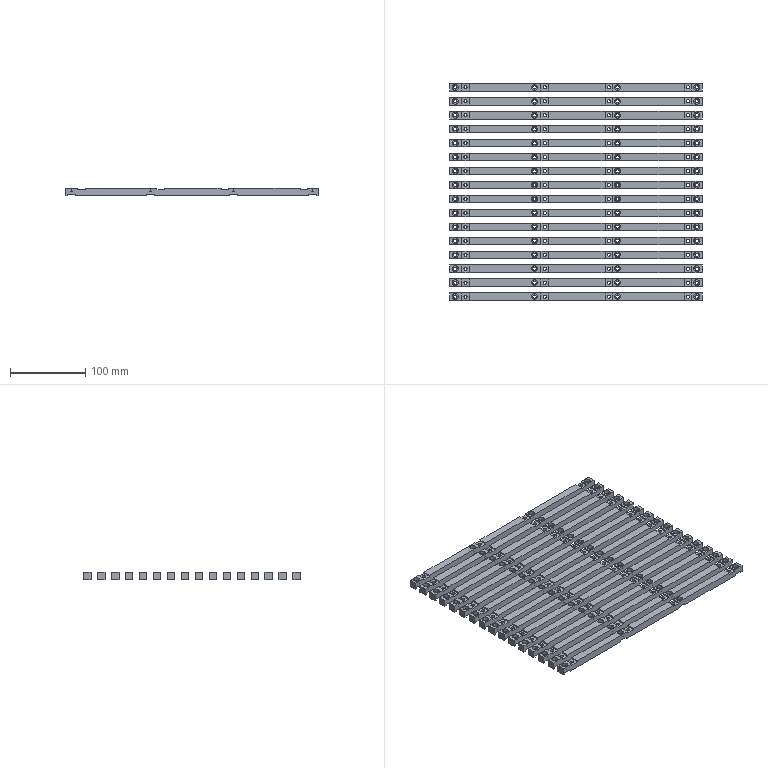CAM job | NX | 3-axis milling, drilling | part box 335 x 287.5 x 10 mm | stock box 341 x 293.5 x 11 mm
Tools:
number,name,description,diameter,corner_radius,flute_length,length,flutes
1,D63,Milling Tool-5 Parameters,63.0,0.0,50.0,75.0,2
7,D6A45,Milling Tool-5 Parameters,6.0,0.0,3.0,3.0,2
14,4.2ZT,Drilling Tool,4.2,0.0,35.0,50.0,2
15,M5,Milling Tool-5 Parameters,4.2,0.0,30.0,30.0,4
17,4.5ZT,Drilling Tool,4.5,0.0,35.0,50.0,2
6,D6,Milling Tool-5 Parameters,6.0,0.0,50.0,75.0,2
4,D4,Milling Tool-5 Parameters,4.0,0.0,50.0,75.0,2
Operations:
program,operation,operation_type,tool,method,geometry_group,spindle_rpm,surface_speed,feed_per_tooth,feed_cut,feed_plunge,cut_length_mm,path_length_mm,cut_time_min,machine_time_min
1-335-293-10毛胚AB胶,FLOOR_WALL,VolumeBased25DMillingOperation,D63,METHOD,A,6500.0,1286.0,0.0962,1250.0,100.0,4320.297,4374.297,3.456,3.462
1-335-293-10毛胚AB胶,DRILLING_COPY_1,Operation,D6A45,METHOD,A,3000.0,56.0,0.0333,200.0,0.0,40.8,484.179,0.204,0.2483
1-335-293-10毛胚AB胶,DRILLING_COPY_1_COPY,Operation,4.2ZT,METHOD,A,2000.0,15.0,0.0375,150.0,0.0,63.047,490.233,0.4203,0.463
1-335-293-10毛胚AB胶,DRILLING_COPY_1_COPY_COPY_1,Operation,4.2ZT,METHOD,A,2000.0,15.0,0.0375,150.0,0.0,63.047,490.233,0.4203,0.463
1-335-293-10毛胚AB胶,DRILLING_COPY_1_COPY_COPY_2,Operation,4.2ZT,METHOD,A,2000.0,15.0,0.0375,150.0,0.0,63.047,490.233,0.4203,0.463
1-335-293-10毛胚AB胶,DRILLING_COPY_1_COPY_COPY_3,Operation,4.2ZT,METHOD,A,2000.0,15.0,0.0375,150.0,0.0,63.047,490.233,0.4203,0.463
1-335-293-10毛胚AB胶,DRILLING_COPY_1_COPY_COPY_4,Operation,4.2ZT,METHOD,A,2000.0,15.0,0.0375,150.0,0.0,63.047,490.233,0.4203,0.463
1-335-293-10毛胚AB胶,DRILLING_COPY_1_COPY_COPY_5,Operation,4.2ZT,METHOD,A,2000.0,15.0,0.0375,150.0,0.0,63.047,490.233,0.4203,0.463
1-335-293-10毛胚AB胶,DRILLING_COPY_1_COPY_COPY_6,Operation,4.2ZT,METHOD,A,2000.0,15.0,0.0375,150.0,0.0,63.047,490.233,0.4203,0.463
1-335-293-10毛胚AB胶,DRILLING_COPY_1_COPY_COPY_7,Operation,4.2ZT,METHOD,A,2000.0,15.0,0.0375,150.0,0.0,63.047,490.233,0.4203,0.463
1-335-293-10毛胚AB胶,DRILLING_COPY_1_COPY_COPY_8,Operation,4.2ZT,METHOD,A,2000.0,15.0,0.0375,150.0,0.0,63.047,490.233,0.4203,0.463
1-335-293-10毛胚AB胶,DRILLING_COPY_1_COPY_COPY_9,Operation,4.2ZT,METHOD,A,2000.0,15.0,0.0375,150.0,0.0,63.047,490.233,0.4203,0.463
1-335-293-10毛胚AB胶,DRILLING_COPY_1_COPY_COPY_10,Operation,4.2ZT,METHOD,A,2000.0,15.0,0.0375,150.0,0.0,63.047,490.233,0.4203,0.463
1-335-293-10毛胚AB胶,DRILLING_COPY_1_COPY_COPY_11,Operation,4.2ZT,METHOD,A,2000.0,15.0,0.0375,150.0,0.0,63.047,490.233,0.4203,0.463
1-335-293-10毛胚AB胶,DRILLING_COPY_1_COPY_COPY_12,Operation,4.2ZT,METHOD,A,2000.0,15.0,0.0375,150.0,0.0,63.047,490.233,0.4203,0.463
1-335-293-10毛胚AB胶,DRILLING_COPY_1_COPY_COPY_13,Operation,4.2ZT,METHOD,A,2000.0,15.0,0.0375,150.0,0.0,63.047,490.233,0.4203,0.463
1-335-293-10毛胚AB胶,DRILLING_COPY_1_COPY_COPY_14,Operation,4.2ZT,METHOD,A,2000.0,15.0,0.0375,150.0,0.0,63.047,490.233,0.4203,0.463
1-335-293-10毛胚AB胶,DRILLING_COPY_1_COPY_COPY_15,Operation,4.2ZT,METHOD,A,2000.0,15.0,0.0375,150.0,0.0,63.047,490.233,0.4203,0.463
1-335-293-10毛胚AB胶,DRILLING_COPY_1_COPY_COPY,Operation,M5,METHOD,A,200.0,2.0,0.2,160.0,0.0,54.0,472.139,0.3375,0.3793
1-335-293-10毛胚AB胶,DRILLING_COPY_1_COPY_COPY_COPY,Operation,M5,METHOD,A,200.0,2.0,0.2,160.0,0.0,54.0,472.139,0.3375,0.3793
1-335-293-10毛胚AB胶,DRILLING_COPY_1_COPY_COPY_COPY_1,Operation,M5,METHOD,A,200.0,2.0,0.2,160.0,0.0,54.0,472.139,0.3375,0.3793
1-335-293-10毛胚AB胶,DRILLING_COPY_1_COPY_COPY_COPY_2,Operation,M5,METHOD,A,200.0,2.0,0.2,160.0,0.0,54.0,472.139,0.3375,0.3793
1-335-293-10毛胚AB胶,DRILLING_COPY_1_COPY_COPY_COPY_3,Operation,M5,METHOD,A,200.0,2.0,0.2,160.0,0.0,54.0,472.139,0.3375,0.3793
1-335-293-10毛胚AB胶,DRILLING_COPY_1_COPY_COPY_COPY_4,Operation,M5,METHOD,A,200.0,2.0,0.2,160.0,0.0,54.0,472.139,0.3375,0.3793
1-335-293-10毛胚AB胶,DRILLING_COPY_1_COPY_COPY_COPY_5,Operation,M5,METHOD,A,200.0,2.0,0.2,160.0,0.0,54.0,472.139,0.3375,0.3793
1-335-293-10毛胚AB胶,DRILLING_COPY_1_COPY_COPY_COPY_6,Operation,M5,METHOD,A,200.0,2.0,0.2,160.0,0.0,54.0,472.139,0.3375,0.3793
1-335-293-10毛胚AB胶,DRILLING_COPY_1_COPY_COPY_COPY_7,Operation,M5,METHOD,A,200.0,2.0,0.2,160.0,0.0,54.0,472.139,0.3375,0.3793
1-335-293-10毛胚AB胶,DRILLING_COPY_1_COPY_COPY_COPY_8,Operation,M5,METHOD,A,200.0,2.0,0.2,160.0,0.0,54.0,472.139,0.3375,0.3793
1-335-293-10毛胚AB胶,DRILLING_COPY_1_COPY_COPY_COPY_9,Operation,M5,METHOD,A,200.0,2.0,0.2,160.0,0.0,54.0,472.139,0.3375,0.3793
1-335-293-10毛胚AB胶,DRILLING_COPY_1_COPY_COPY_COPY_10,Operation,M5,METHOD,A,200.0,2.0,0.2,160.0,0.0,54.0,472.139,0.3375,0.3793
1-335-293-10毛胚AB胶,DRILLING_COPY_1_COPY_COPY_COPY_11,Operation,M5,METHOD,A,200.0,2.0,0.2,160.0,0.0,54.0,472.139,0.3375,0.3793
1-335-293-10毛胚AB胶,DRILLING_COPY_1_COPY_COPY_COPY_12,Operation,M5,METHOD,A,200.0,2.0,0.2,160.0,0.0,54.0,472.139,0.3375,0.3793
1-335-293-10毛胚AB胶,DRILLING_COPY_1_COPY_COPY_COPY_13,Operation,M5,METHOD,A,200.0,2.0,0.2,160.0,0.0,54.0,472.139,0.3375,0.3793
1-335-293-10毛胚AB胶,DRILLING_COPY_1_COPY_COPY_COPY_14,Operation,M5,METHOD,A,200.0,2.0,0.2,160.0,0.0,54.0,472.139,0.3375,0.3793
1-335-293-10毛胚AB胶,DRILLING_COPY_1_COPY_COPY_16,Operation,4.5ZT,METHOD,A,2000.0,28.0,0.0375,150.0,0.0,55.408,499.942,0.3694,0.4138
1-335-293-10毛胚AB胶,DRILLING_COPY_1_COPY_COPY_16_COPY,Operation,4.5ZT,METHOD,A,2000.0,28.0,0.0375,150.0,0.0,55.408,499.942,0.3694,0.4138
1-335-293-10毛胚AB胶,DRILLING_COPY_1_COPY_COPY_16_COPY_1,Operation,4.5ZT,METHOD,A,2000.0,28.0,0.0375,150.0,0.0,55.408,499.942,0.3694,0.4138
1-335-293-10毛胚AB胶,DRILLING_COPY_1_COPY_COPY_16_COPY_2,Operation,4.5ZT,METHOD,A,2000.0,28.0,0.0375,150.0,0.0,55.408,499.942,0.3694,0.4138
1-335-293-10毛胚AB胶,DRILLING_COPY_1_COPY_COPY_16_COPY_3,Operation,4.5ZT,METHOD,A,2000.0,28.0,0.0375,150.0,0.0,55.408,499.942,0.3694,0.4138
1-335-293-10毛胚AB胶,DRILLING_COPY_1_COPY_COPY_16_COPY_4,Operation,4.5ZT,METHOD,A,2000.0,28.0,0.0375,150.0,0.0,55.408,499.942,0.3694,0.4138
1-335-293-10毛胚AB胶,DRILLING_COPY_1_COPY_COPY_16_COPY_5,Operation,4.5ZT,METHOD,A,2000.0,28.0,0.0375,150.0,0.0,55.408,499.942,0.3694,0.4138
1-335-293-10毛胚AB胶,DRILLING_COPY_1_COPY_COPY_16_COPY_6,Operation,4.5ZT,METHOD,A,2000.0,28.0,0.0375,150.0,0.0,55.408,499.942,0.3694,0.4138
1-335-293-10毛胚AB胶,DRILLING_COPY_1_COPY_COPY_16_COPY_7,Operation,4.5ZT,METHOD,A,2000.0,28.0,0.0375,150.0,0.0,55.408,499.942,0.3694,0.4138
1-335-293-10毛胚AB胶,DRILLING_COPY_1_COPY_COPY_16_COPY_8,Operation,4.5ZT,METHOD,A,2000.0,28.0,0.0375,150.0,0.0,55.408,499.942,0.3694,0.4138
1-335-293-10毛胚AB胶,DRILLING_COPY_1_COPY_COPY_16_COPY_9,Operation,4.5ZT,METHOD,A,2000.0,28.0,0.0375,150.0,0.0,55.408,499.942,0.3694,0.4138
1-335-293-10毛胚AB胶,DRILLING_COPY_1_COPY_COPY_16_COPY_10,Operation,4.5ZT,METHOD,A,2000.0,28.0,0.0375,150.0,0.0,55.408,499.942,0.3694,0.4138
1-335-293-10毛胚AB胶,DRILLING_COPY_1_COPY_COPY_16_COPY_11,Operation,4.5ZT,METHOD,A,2000.0,28.0,0.0375,150.0,0.0,55.408,499.942,0.3694,0.4138
1-335-293-10毛胚AB胶,DRILLING_COPY_1_COPY_COPY_16_COPY_12,Operation,4.5ZT,METHOD,A,2000.0,28.0,0.0375,150.0,0.0,55.408,499.942,0.3694,0.4138
1-335-293-10毛胚AB胶,DRILLING_COPY_1_COPY_COPY_16_COPY_13,Operation,4.5ZT,METHOD,A,2000.0,28.0,0.0375,150.0,0.0,55.408,499.942,0.3694,0.4138
1-335-293-10毛胚AB胶,DRILLING_COPY_1_COPY_COPY_16_COPY_14,Operation,4.5ZT,METHOD,A,2000.0,28.0,0.0375,150.0,0.0,55.408,499.942,0.3694,0.4138
1-335-293-10毛胚AB胶,HOLE_MILLING,CylinderMilling,D6,METHOD,A,7000.0,131.0,0.1071,1500.0,100.0,5539.175,11188.331,3.693,4.258
1-335-293-10毛胚AB胶,ZLEVEL_PROFILE,ZLevelMilling,D6,METHOD,A,7000.0,219.0,0.2143,3000.0,1000.0,273402.094,275716.326,91.52,91.751
1-335-293-10毛胚AB胶,ZLEVEL_PROFILE_COPY,ZLevelMilling,D6,METHOD,A,7000.0,219.0,0.1429,2000.0,1000.0,11936.828,12762.929,5.987,6.07
1-335-293-10毛胚AB胶,ZLEVEL_PROFILE_COPY_1_COPY_COPY_COPY_COPY_2_COPY,ZLevelMilling,D6A45,METHOD,A,7000.0,131.0,0.0714,1000.0,1000.0,13308.137,42962.116,13.308,16.273
1-335-293-10毛胚AB胶,刀补6,ZLevelMilling,D4,METHOD,A,7000.0,219.0,0.0714,1000.0,1000.0,2380.142,3189.749,2.38,2.461
1-335-293-10毛胚AB胶,ZLEVEL_PROFILE_COPY_1_1,ZLevelMilling,D6,METHOD,A,7000.0,219.0,0.0714,1000.0,1000.0,34669.721,39627.299,34.67,35.166